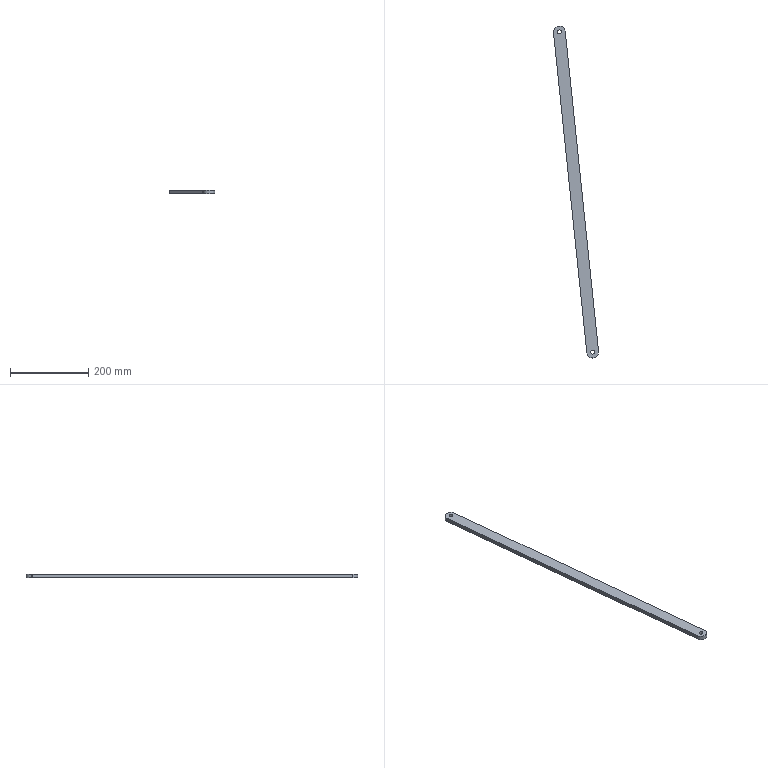Part | SolidWorks | features Extrusion 1 | 1 solid | 11 faces | box 115.162 x 846.43 x 10 mm | volume 253110 mm3 | cylinder 7 | plane 4 | commonest cylinder face diameters 10 x4 30.162 x3
STEP:
#1=CARTESIAN_POINT('',(80.,-18.24,10.));
#2=VERTEX_POINT('',#1);
#3=CARTESIAN_POINT('',(90.,-18.24,10.));
#4=VERTEX_POINT('',#3);
#5=CARTESIAN_POINT('',(85.,-18.24,10.));
#6=DIRECTION('',(0.,0.,1.));
#7=DIRECTION('',(1.,0.,0.));
#8=AXIS2_PLACEMENT_3D('',#5,#6,#7);
#9=CIRCLE('',#8,5.);
#10=EDGE_CURVE('',#2,#4,#9,.T.);
#11=ORIENTED_EDGE('',*,*,#10,.T.);
#12=CARTESIAN_POINT('',(90.,-18.24,0.));
#13=VERTEX_POINT('',#12);
#14=CARTESIAN_POINT('',(90.,-18.24,10.));
#15=DIRECTION('',(0.,0.,-1.));
#16=VECTOR('',#15,1000.);
#17=LINE('',#14,#16);
#18=EDGE_CURVE('',#4,#13,#17,.T.);
#19=ORIENTED_EDGE('',*,*,#18,.T.);
#20=CARTESIAN_POINT('',(80.,-18.24,0.));
#21=VERTEX_POINT('',#20);
#22=CARTESIAN_POINT('',(85.,-18.24,0.));
#23=DIRECTION('',(0.,0.,1.));
#24=DIRECTION('',(1.,0.,0.));
#25=AXIS2_PLACEMENT_3D('',#22,#23,#24);
#26=CIRCLE('',#25,5.);
#27=EDGE_CURVE('',#21,#13,#26,.T.);
#28=ORIENTED_EDGE('',*,*,#27,.F.);
#29=CARTESIAN_POINT('',(80.,-18.24,10.));
#30=DIRECTION('',(0.,0.,-1.));
#31=VECTOR('',#30,1000.);
#32=LINE('',#29,#31);
#33=EDGE_CURVE('',#2,#21,#32,.T.);
#34=ORIENTED_EDGE('',*,*,#33,.F.);
#35=EDGE_LOOP('',(#11,#19,#28,#34));
#36=FACE_OUTER_BOUND('',#35,.T.);
#37=CARTESIAN_POINT('',(85.,-18.24,10.));
#38=DIRECTION('',(0.,0.,-1.));
#39=DIRECTION('',(-1.,0.,0.));
#40=AXIS2_PLACEMENT_3D('',#37,#38,#39);
#41=CYLINDRICAL_SURFACE('',#40,5.);
#42=ADVANCED_FACE('',(#36),#41,.F.);
#43=CARTESIAN_POINT('',(-5.,798.028,10.));
#44=VERTEX_POINT('',#43);
#45=CARTESIAN_POINT('',(5.,798.028,10.));
#46=VERTEX_POINT('',#45);
#47=CARTESIAN_POINT('',(0.,798.028,10.));
#48=DIRECTION('',(0.,0.,1.));
#49=DIRECTION('',(1.,0.,0.));
#50=AXIS2_PLACEMENT_3D('',#47,#48,#49);
#51=CIRCLE('',#50,5.);
#52=EDGE_CURVE('',#44,#46,#51,.T.);
#53=ORIENTED_EDGE('',*,*,#52,.T.);
#54=CARTESIAN_POINT('',(5.,798.028,0.));
#55=VERTEX_POINT('',#54);
#56=CARTESIAN_POINT('',(5.,798.028,10.));
#57=DIRECTION('',(0.,0.,-1.));
#58=VECTOR('',#57,1000.);
#59=LINE('',#56,#58);
#60=EDGE_CURVE('',#46,#55,#59,.T.);
#61=ORIENTED_EDGE('',*,*,#60,.T.);
#62=CARTESIAN_POINT('',(-5.,798.028,0.));
#63=VERTEX_POINT('',#62);
#64=CARTESIAN_POINT('',(0.,798.028,0.));
#65=DIRECTION('',(0.,0.,1.));
#66=DIRECTION('',(1.,0.,0.));
#67=AXIS2_PLACEMENT_3D('',#64,#65,#66);
#68=CIRCLE('',#67,5.);
#69=EDGE_CURVE('',#63,#55,#68,.T.);
#70=ORIENTED_EDGE('',*,*,#69,.F.);
#71=CARTESIAN_POINT('',(-5.,798.028,10.));
#72=DIRECTION('',(0.,0.,-1.));
#73=VECTOR('',#72,1000.);
#74=LINE('',#71,#73);
#75=EDGE_CURVE('',#44,#63,#74,.T.);
#76=ORIENTED_EDGE('',*,*,#75,.F.);
#77=EDGE_LOOP('',(#53,#61,#70,#76));
#78=FACE_OUTER_BOUND('',#77,.T.);
#79=CARTESIAN_POINT('',(0.,798.028,10.));
#80=DIRECTION('',(0.,0.,-1.));
#81=DIRECTION('',(-1.,0.,0.));
#82=AXIS2_PLACEMENT_3D('',#79,#80,#81);
#83=CYLINDRICAL_SURFACE('',#82,5.);
#84=ADVANCED_FACE('',(#78),#83,.F.);
#85=CARTESIAN_POINT('',(-15.081,798.028,10.));
#86=VERTEX_POINT('',#85);
#87=CARTESIAN_POINT('',(-15.,796.466,10.));
#88=VERTEX_POINT('',#87);
#89=CARTESIAN_POINT('',(0.,798.028,10.));
#90=DIRECTION('',(0.,0.,1.));
#91=DIRECTION('',(1.,0.,0.));
#92=AXIS2_PLACEMENT_3D('',#89,#90,#91);
#93=CIRCLE('',#92,15.081);
#94=EDGE_CURVE('',#86,#88,#93,.T.);
#95=ORIENTED_EDGE('',*,*,#94,.F.);
#96=CARTESIAN_POINT('',(-15.081,798.028,0.));
#97=VERTEX_POINT('',#96);
#98=CARTESIAN_POINT('',(-15.081,798.028,10.));
#99=DIRECTION('',(0.,0.,-1.));
#100=VECTOR('',#99,1000.);
#101=LINE('',#98,#100);
#102=EDGE_CURVE('',#86,#97,#101,.T.);
#103=ORIENTED_EDGE('',*,*,#102,.T.);
#104=CARTESIAN_POINT('',(-15.,796.466,0.));
#105=VERTEX_POINT('',#104);
#106=CARTESIAN_POINT('',(0.,798.028,0.));
#107=DIRECTION('',(0.,0.,1.));
#108=DIRECTION('',(1.,0.,0.));
#109=AXIS2_PLACEMENT_3D('',#106,#107,#108);
#110=CIRCLE('',#109,15.081);
#111=EDGE_CURVE('',#97,#105,#110,.T.);
#112=ORIENTED_EDGE('',*,*,#111,.T.);
#113=CARTESIAN_POINT('',(-15.,796.466,10.));
#114=DIRECTION('',(0.,0.,-1.));
#115=VECTOR('',#114,1000.);
#116=LINE('',#113,#115);
#117=EDGE_CURVE('',#88,#105,#116,.T.);
#118=ORIENTED_EDGE('',*,*,#117,.F.);
#119=EDGE_LOOP('',(#95,#103,#112,#118));
#120=FACE_OUTER_BOUND('',#119,.T.);
#121=CARTESIAN_POINT('',(0.,798.028,10.));
#122=DIRECTION('',(0.,0.,-1.));
#123=DIRECTION('',(-1.,0.,0.));
#124=AXIS2_PLACEMENT_3D('',#121,#122,#123);
#125=CYLINDRICAL_SURFACE('',#124,15.081);
#126=ADVANCED_FACE('',(#120),#125,.T.);
#127=ORIENTED_EDGE('',*,*,#52,.F.);
#128=CARTESIAN_POINT('',(0.,798.028,10.));
#129=DIRECTION('',(0.,0.,1.));
#130=DIRECTION('',(1.,0.,0.));
#131=AXIS2_PLACEMENT_3D('',#128,#129,#130);
#132=CIRCLE('',#131,5.);
#133=EDGE_CURVE('',#46,#44,#132,.T.);
#134=ORIENTED_EDGE('',*,*,#133,.F.);
#135=EDGE_LOOP('',(#127,#134));
#136=FACE_BOUND('',#135,.T.);
#137=CARTESIAN_POINT('',(70.,-19.802,10.));
#138=VERTEX_POINT('',#137);
#139=CARTESIAN_POINT('',(100.,-16.678,10.));
#140=VERTEX_POINT('',#139);
#141=CARTESIAN_POINT('',(85.,-18.24,10.));
#142=DIRECTION('',(0.,0.,1.));
#143=DIRECTION('',(1.,0.,0.));
#144=AXIS2_PLACEMENT_3D('',#141,#142,#143);
#145=CIRCLE('',#144,15.081);
#146=EDGE_CURVE('',#138,#140,#145,.T.);
#147=ORIENTED_EDGE('',*,*,#146,.T.);
#148=CARTESIAN_POINT('',(15.,799.59,10.));
#149=VERTEX_POINT('',#148);
#150=CARTESIAN_POINT('',(100.,-16.678,10.));
#151=DIRECTION('',(-0.1036,0.9946,0.));
#152=VECTOR('',#151,1000.);
#153=LINE('',#150,#152);
#154=EDGE_CURVE('',#140,#149,#153,.T.);
#155=ORIENTED_EDGE('',*,*,#154,.T.);
#156=CARTESIAN_POINT('',(0.,798.028,10.));
#157=DIRECTION('',(0.,0.,1.));
#158=DIRECTION('',(1.,0.,0.));
#159=AXIS2_PLACEMENT_3D('',#156,#157,#158);
#160=CIRCLE('',#159,15.081);
#161=EDGE_CURVE('',#149,#86,#160,.T.);
#162=ORIENTED_EDGE('',*,*,#161,.T.);
#163=ORIENTED_EDGE('',*,*,#94,.T.);
#164=CARTESIAN_POINT('',(-15.,796.466,10.));
#165=DIRECTION('',(0.1036,-0.9946,0.));
#166=VECTOR('',#165,1000.);
#167=LINE('',#164,#166);
#168=EDGE_CURVE('',#88,#138,#167,.T.);
#169=ORIENTED_EDGE('',*,*,#168,.T.);
#170=EDGE_LOOP('',(#147,#155,#162,#163,#169));
#171=FACE_OUTER_BOUND('',#170,.T.);
#172=ORIENTED_EDGE('',*,*,#10,.F.);
#173=CARTESIAN_POINT('',(85.,-18.24,10.));
#174=DIRECTION('',(0.,0.,1.));
#175=DIRECTION('',(1.,0.,0.));
#176=AXIS2_PLACEMENT_3D('',#173,#174,#175);
#177=CIRCLE('',#176,5.);
#178=EDGE_CURVE('',#4,#2,#177,.T.);
#179=ORIENTED_EDGE('',*,*,#178,.F.);
#180=EDGE_LOOP('',(#172,#179));
#181=FACE_BOUND('',#180,.T.);
#182=CARTESIAN_POINT('',(85.,-18.24,10.));
#183=DIRECTION('',(0.,0.,1.));
#184=DIRECTION('',(1.,0.,0.));
#185=AXIS2_PLACEMENT_3D('',#182,#183,#184);
#186=PLANE('',#185);
#187=ADVANCED_FACE('',(#136,#171,#181),#186,.T.);
#188=CARTESIAN_POINT('',(70.,-19.802,0.));
#189=VERTEX_POINT('',#188);
#190=CARTESIAN_POINT('',(100.,-16.678,0.));
#191=VERTEX_POINT('',#190);
#192=CARTESIAN_POINT('',(85.,-18.24,0.));
#193=DIRECTION('',(0.,0.,1.));
#194=DIRECTION('',(1.,0.,0.));
#195=AXIS2_PLACEMENT_3D('',#192,#193,#194);
#196=CIRCLE('',#195,15.081);
#197=EDGE_CURVE('',#189,#191,#196,.T.);
#198=ORIENTED_EDGE('',*,*,#197,.F.);
#199=CARTESIAN_POINT('',(-15.,796.466,0.));
#200=DIRECTION('',(0.1036,-0.9946,0.));
#201=VECTOR('',#200,1000.);
#202=LINE('',#199,#201);
#203=EDGE_CURVE('',#105,#189,#202,.T.);
#204=ORIENTED_EDGE('',*,*,#203,.F.);
#205=ORIENTED_EDGE('',*,*,#111,.F.);
#206=CARTESIAN_POINT('',(15.,799.59,0.));
#207=VERTEX_POINT('',#206);
#208=CARTESIAN_POINT('',(0.,798.028,0.));
#209=DIRECTION('',(0.,0.,1.));
#210=DIRECTION('',(1.,0.,0.));
#211=AXIS2_PLACEMENT_3D('',#208,#209,#210);
#212=CIRCLE('',#211,15.081);
#213=EDGE_CURVE('',#207,#97,#212,.T.);
#214=ORIENTED_EDGE('',*,*,#213,.F.);
#215=CARTESIAN_POINT('',(100.,-16.678,0.));
#216=DIRECTION('',(-0.1036,0.9946,0.));
#217=VECTOR('',#216,1000.);
#218=LINE('',#215,#217);
#219=EDGE_CURVE('',#191,#207,#218,.T.);
#220=ORIENTED_EDGE('',*,*,#219,.F.);
#221=EDGE_LOOP('',(#198,#204,#205,#214,#220));
#222=FACE_OUTER_BOUND('',#221,.T.);
#223=ORIENTED_EDGE('',*,*,#69,.T.);
#224=CARTESIAN_POINT('',(0.,798.028,0.));
#225=DIRECTION('',(0.,0.,1.));
#226=DIRECTION('',(1.,0.,0.));
#227=AXIS2_PLACEMENT_3D('',#224,#225,#226);
#228=CIRCLE('',#227,5.);
#229=EDGE_CURVE('',#55,#63,#228,.T.);
#230=ORIENTED_EDGE('',*,*,#229,.T.);
#231=EDGE_LOOP('',(#223,#230));
#232=FACE_BOUND('',#231,.T.);
#233=ORIENTED_EDGE('',*,*,#27,.T.);
#234=CARTESIAN_POINT('',(85.,-18.24,0.));
#235=DIRECTION('',(0.,0.,1.));
#236=DIRECTION('',(1.,0.,0.));
#237=AXIS2_PLACEMENT_3D('',#234,#235,#236);
#238=CIRCLE('',#237,5.);
#239=EDGE_CURVE('',#13,#21,#238,.T.);
#240=ORIENTED_EDGE('',*,*,#239,.T.);
#241=EDGE_LOOP('',(#233,#240));
#242=FACE_BOUND('',#241,.T.);
#243=CARTESIAN_POINT('',(85.,-18.24,0.));
#244=DIRECTION('',(0.,0.,1.));
#245=DIRECTION('',(1.,0.,0.));
#246=AXIS2_PLACEMENT_3D('',#243,#244,#245);
#247=PLANE('',#246);
#248=ADVANCED_FACE('',(#222,#232,#242),#247,.F.);
#249=ORIENTED_EDGE('',*,*,#197,.T.);
#250=CARTESIAN_POINT('',(100.,-16.678,10.));
#251=DIRECTION('',(0.,0.,-1.));
#252=VECTOR('',#251,1000.);
#253=LINE('',#250,#252);
#254=EDGE_CURVE('',#140,#191,#253,.T.);
#255=ORIENTED_EDGE('',*,*,#254,.F.);
#256=ORIENTED_EDGE('',*,*,#146,.F.);
#257=CARTESIAN_POINT('',(70.,-19.802,10.));
#258=DIRECTION('',(0.,0.,-1.));
#259=VECTOR('',#258,1000.);
#260=LINE('',#257,#259);
#261=EDGE_CURVE('',#138,#189,#260,.T.);
#262=ORIENTED_EDGE('',*,*,#261,.T.);
#263=EDGE_LOOP('',(#249,#255,#256,#262));
#264=FACE_OUTER_BOUND('',#263,.T.);
#265=CARTESIAN_POINT('',(85.,-18.24,10.));
#266=DIRECTION('',(0.,0.,-1.));
#267=DIRECTION('',(-1.,0.,0.));
#268=AXIS2_PLACEMENT_3D('',#265,#266,#267);
#269=CYLINDRICAL_SURFACE('',#268,15.081);
#270=ADVANCED_FACE('',(#264),#269,.T.);
#271=ORIENTED_EDGE('',*,*,#219,.T.);
#272=CARTESIAN_POINT('',(15.,799.59,10.));
#273=DIRECTION('',(0.,0.,-1.));
#274=VECTOR('',#273,1000.);
#275=LINE('',#272,#274);
#276=EDGE_CURVE('',#149,#207,#275,.T.);
#277=ORIENTED_EDGE('',*,*,#276,.F.);
#278=ORIENTED_EDGE('',*,*,#154,.F.);
#279=ORIENTED_EDGE('',*,*,#254,.T.);
#280=EDGE_LOOP('',(#271,#277,#278,#279));
#281=FACE_OUTER_BOUND('',#280,.T.);
#282=CARTESIAN_POINT('',(100.,-16.678,10.));
#283=DIRECTION('',(-0.9946,-0.1036,0.));
#284=DIRECTION('',(0.1036,-0.9946,0.));
#285=AXIS2_PLACEMENT_3D('',#282,#283,#284);
#286=PLANE('',#285);
#287=ADVANCED_FACE('',(#281),#286,.F.);
#288=ORIENTED_EDGE('',*,*,#102,.F.);
#289=ORIENTED_EDGE('',*,*,#161,.F.);
#290=ORIENTED_EDGE('',*,*,#276,.T.);
#291=ORIENTED_EDGE('',*,*,#213,.T.);
#292=EDGE_LOOP('',(#288,#289,#290,#291));
#293=FACE_OUTER_BOUND('',#292,.T.);
#294=CARTESIAN_POINT('',(0.,798.028,10.));
#295=DIRECTION('',(0.,0.,-1.));
#296=DIRECTION('',(-1.,0.,0.));
#297=AXIS2_PLACEMENT_3D('',#294,#295,#296);
#298=CYLINDRICAL_SURFACE('',#297,15.081);
#299=ADVANCED_FACE('',(#293),#298,.T.);
#300=ORIENTED_EDGE('',*,*,#203,.T.);
#301=ORIENTED_EDGE('',*,*,#261,.F.);
#302=ORIENTED_EDGE('',*,*,#168,.F.);
#303=ORIENTED_EDGE('',*,*,#117,.T.);
#304=EDGE_LOOP('',(#300,#301,#302,#303));
#305=FACE_OUTER_BOUND('',#304,.T.);
#306=CARTESIAN_POINT('',(-15.,796.466,10.));
#307=DIRECTION('',(0.9946,0.1036,0.));
#308=DIRECTION('',(-0.1036,0.9946,0.));
#309=AXIS2_PLACEMENT_3D('',#306,#307,#308);
#310=PLANE('',#309);
#311=ADVANCED_FACE('',(#305),#310,.F.);
#312=ORIENTED_EDGE('',*,*,#60,.F.);
#313=ORIENTED_EDGE('',*,*,#133,.T.);
#314=ORIENTED_EDGE('',*,*,#75,.T.);
#315=ORIENTED_EDGE('',*,*,#229,.F.);
#316=EDGE_LOOP('',(#312,#313,#314,#315));
#317=FACE_OUTER_BOUND('',#316,.T.);
#318=CARTESIAN_POINT('',(0.,798.028,10.));
#319=DIRECTION('',(0.,0.,-1.));
#320=DIRECTION('',(-1.,0.,0.));
#321=AXIS2_PLACEMENT_3D('',#318,#319,#320);
#322=CYLINDRICAL_SURFACE('',#321,5.);
#323=ADVANCED_FACE('',(#317),#322,.F.);
#324=ORIENTED_EDGE('',*,*,#18,.F.);
#325=ORIENTED_EDGE('',*,*,#178,.T.);
#326=ORIENTED_EDGE('',*,*,#33,.T.);
#327=ORIENTED_EDGE('',*,*,#239,.F.);
#328=EDGE_LOOP('',(#324,#325,#326,#327));
#329=FACE_OUTER_BOUND('',#328,.T.);
#330=CARTESIAN_POINT('',(85.,-18.24,10.));
#331=DIRECTION('',(0.,0.,-1.));
#332=DIRECTION('',(-1.,0.,0.));
#333=AXIS2_PLACEMENT_3D('',#330,#331,#332);
#334=CYLINDRICAL_SURFACE('',#333,5.);
#335=ADVANCED_FACE('',(#329),#334,.F.);
#336=CLOSED_SHELL('',(#42,#84,#126,#187,#248,#270,#287,#299,#311,#323,#335));
#337=MANIFOLD_SOLID_BREP('',#336);
#338=CARTESIAN_POINT('',(0.,0.,0.));
#339=DIRECTION('',(0.,0.,1.));
#340=DIRECTION('',(1.,0.,0.));
#341=AXIS2_PLACEMENT_3D('',#338,#339,#340);
#342=(LENGTH_UNIT()NAMED_UNIT(*)SI_UNIT(.MILLI.,.METRE.));
#343=UNCERTAINTY_MEASURE_WITH_UNIT(LENGTH_MEASURE(0.00001),#342,'','');
#344=(NAMED_UNIT(*)PLANE_ANGLE_UNIT()SI_UNIT($,.RADIAN.));
#345=(NAMED_UNIT(*)SI_UNIT($,.STERADIAN.)SOLID_ANGLE_UNIT());
#346=(GEOMETRIC_REPRESENTATION_CONTEXT(3)GLOBAL_UNCERTAINTY_ASSIGNED_CONTEXT((#343))GLOBAL_UNIT_ASSIGNED_CONTEXT((#342,#344,#345))REPRESENTATION_CONTEXT('',''));
#347=ADVANCED_BREP_SHAPE_REPRESENTATION('',(#337,#341),#346);